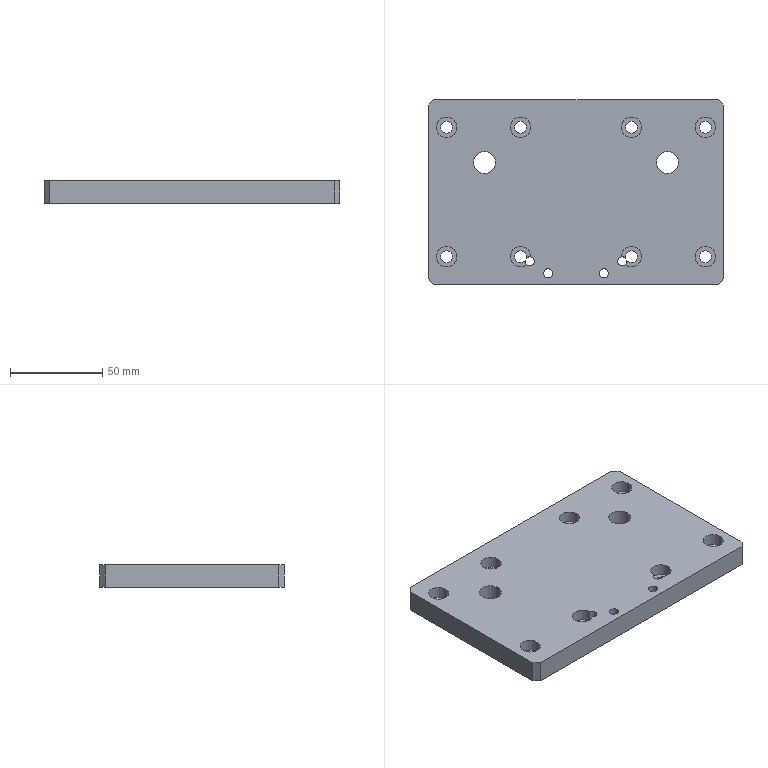Part | SolidWorks | features HoleWzd 4, Chamfer 1, Extrusion 1 | 1 solid | 68 faces | box 160 x 100 x 12 mm | volume 181929 mm3 | cylinder 50 | plane 18 | commonest cylinder face diameters 6.4 x18 11 x18 5 x10 12 x4